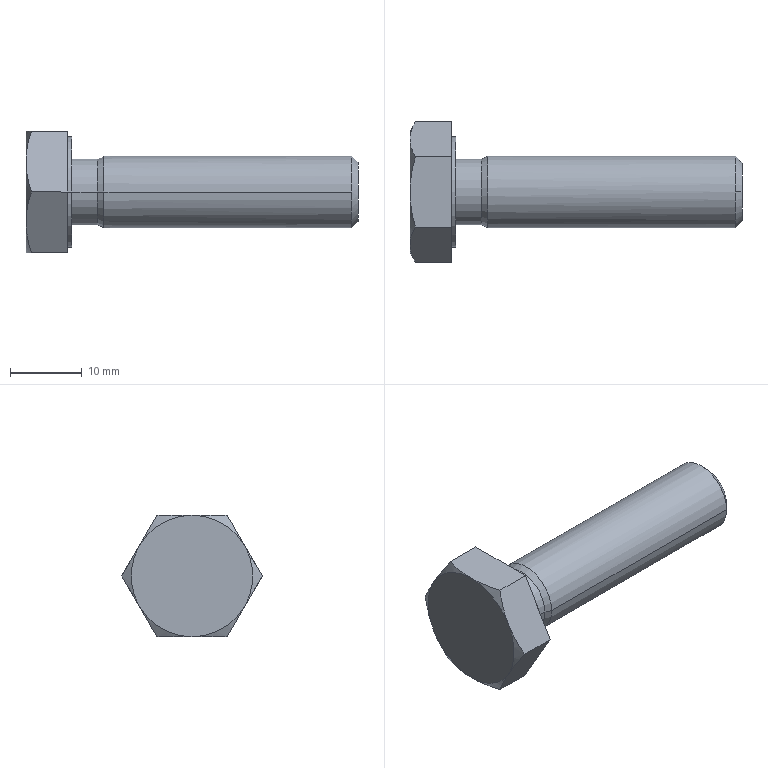Part | STEP file | DIN 933 - replaced by DIN EN 24017 M10  x 40 | 1 solid | 26 faces | box 46.4 x 19.63 x 17 mm | volume 4638 mm3 | cone 10 | plane 10 | cylinder 6 | commonest cylinder face diameters 9.188 x2 10 x2 15.4 x2